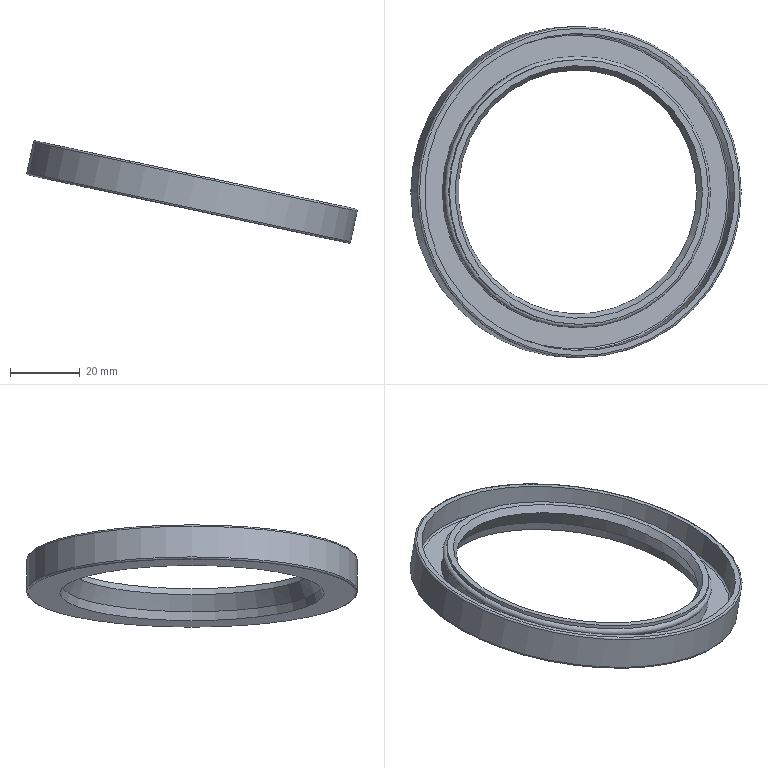Part | STEP file | HL4GZ-1.862.553 (cutter mechanism oil seal) | 1 solid | 15 faces | box 94.817 x 95 x 29.347 mm | volume 14495 mm3 | cone 4 | plane 4 | torus 4 | cylinder 3 | commonest cylinder face diameters 76 x1 91 x1 95 x1
STEP:
#1=CARTESIAN_POINT('',(0.,0.,0.));
#2=DIRECTION('',(0.,0.,1.));
#3=DIRECTION('',(1.,0.,0.));
#4=AXIS2_PLACEMENT_3D('',#1,#2,#3);
#5=CARTESIAN_POINT('',(1986.995,0.00003081,-489.503));
#6=VERTEX_POINT('',#5);
#7=CARTESIAN_POINT('',(1949.826,0.00003081,-481.603));
#8=DIRECTION('',(0.2079,0.,0.9781));
#9=DIRECTION('',(0.9781,0.,-0.2079));
#10=AXIS2_PLACEMENT_3D('',#7,#8,#9);
#11=CIRCLE('',#10,38.);
#12=CARTESIAN_POINT('',(1949.93,0.00003081,-481.114));
#13=DIRECTION('',(0.2079,0.,0.9781));
#14=DIRECTION('',(0.9781,0.,-0.2079));
#15=AXIS2_PLACEMENT_3D('',#12,#13,#14);
#16=CYLINDRICAL_SURFACE('',#15,38.);
#17=CARTESIAN_POINT('',(0.,-0.5));
#18=DIRECTION('',(1.,0.));
#19=VECTOR('',#18,1.);
#20=LINE('',#17,#19);
#21=(GEOMETRIC_REPRESENTATION_CONTEXT(2)PARAMETRIC_REPRESENTATION_CONTEXT()REPRESENTATION_CONTEXT('',''));
#22=DEFINITIONAL_REPRESENTATION('',(#20),#21);
#23=PCURVE('',#16,#22);
#24=CARTESIAN_POINT('',(1949.618,0.00003081,-482.581));
#25=DIRECTION('',(0.2079,0.,0.9781));
#26=DIRECTION('',(0.,-1.,0.));
#27=AXIS2_PLACEMENT_3D('',#24,#25,#26);
#28=TOROIDAL_SURFACE('',#27,38.,1.);
#29=CARTESIAN_POINT('',(1.571,7.854));
#30=DIRECTION('',(1.,0.));
#31=VECTOR('',#30,1.);
#32=LINE('',#29,#31);
#33=(GEOMETRIC_REPRESENTATION_CONTEXT(2)PARAMETRIC_REPRESENTATION_CONTEXT()REPRESENTATION_CONTEXT('',''));
#34=DEFINITIONAL_REPRESENTATION('',(#32),#33);
#35=PCURVE('',#28,#34);
#36=SURFACE_CURVE('',#11,(#23,#35),.PCURVE_S1.);
#37=EDGE_CURVE('',#6,#6,#36,.T.);
#38=ORIENTED_EDGE('',*,*,#37,.T.);
#39=CARTESIAN_POINT('',(1987.203,0.00003081,-488.525));
#40=VERTEX_POINT('',#39);
#41=CARTESIAN_POINT('',(1986.995,0.00003081,-489.503));
#42=CARTESIAN_POINT('',(1987.203,0.00003081,-488.525));
#43=B_SPLINE_CURVE_WITH_KNOTS('',1,(#41,#42),.UNSPECIFIED.,.F.,.F.,(2,2),(-0.5,0.5),.PIECEWISE_BEZIER_KNOTS.);
#44=CARTESIAN_POINT('',(6.283,0.));
#45=DIRECTION('',(0.,1.));
#46=VECTOR('',#45,1.);
#47=LINE('',#44,#46);
#48=(GEOMETRIC_REPRESENTATION_CONTEXT(2)PARAMETRIC_REPRESENTATION_CONTEXT()REPRESENTATION_CONTEXT('',''));
#49=DEFINITIONAL_REPRESENTATION('',(#47),#48);
#50=PCURVE('',#16,#49);
#51=CARTESIAN_POINT('',(0.,0.));
#52=DIRECTION('',(0.,1.));
#53=VECTOR('',#52,1.);
#54=LINE('',#51,#53);
#55=(GEOMETRIC_REPRESENTATION_CONTEXT(2)PARAMETRIC_REPRESENTATION_CONTEXT()REPRESENTATION_CONTEXT('',''));
#56=DEFINITIONAL_REPRESENTATION('',(#54),#55);
#57=PCURVE('',#16,#56);
#58=SEAM_CURVE('',#43,(#50,#57),.PCURVE_S1.);
#59=EDGE_CURVE('',#6,#40,#58,.T.);
#60=ORIENTED_EDGE('',*,*,#59,.T.);
#61=CARTESIAN_POINT('',(1950.034,0.00003081,-480.624));
#62=DIRECTION('',(0.2079,0.,0.9781));
#63=DIRECTION('',(0.9781,0.,-0.2079));
#64=AXIS2_PLACEMENT_3D('',#61,#62,#63);
#65=CIRCLE('',#64,38.);
#66=CARTESIAN_POINT('',(0.,0.5));
#67=DIRECTION('',(1.,0.));
#68=VECTOR('',#67,1.);
#69=LINE('',#66,#68);
#70=(GEOMETRIC_REPRESENTATION_CONTEXT(2)PARAMETRIC_REPRESENTATION_CONTEXT()REPRESENTATION_CONTEXT('',''));
#71=DEFINITIONAL_REPRESENTATION('',(#69),#70);
#72=PCURVE('',#16,#71);
#73=CARTESIAN_POINT('',(1986.347,0.00003081,-488.343));
#74=DIRECTION('',(0.2079,0.,0.9781));
#75=DIRECTION('',(0.,-1.,0.));
#76=AXIS2_PLACEMENT_3D('',#73,#74,#75);
#77=PLANE('',#76);
#78=CARTESIAN_POINT('',(0.,-37.125));
#79=DIRECTION('',(0.,1.));
#80=AXIS2_PLACEMENT_2D('',#78,#79);
#81=CIRCLE('',#80,38.);
#82=(GEOMETRIC_REPRESENTATION_CONTEXT(2)PARAMETRIC_REPRESENTATION_CONTEXT()REPRESENTATION_CONTEXT('',''));
#83=DEFINITIONAL_REPRESENTATION('',(#81),#82);
#84=PCURVE('',#77,#83);
#85=SURFACE_CURVE('',#65,(#72,#84),.PCURVE_S1.);
#86=EDGE_CURVE('',#40,#40,#85,.T.);
#87=ORIENTED_EDGE('',*,*,#86,.F.);
#88=ORIENTED_EDGE('',*,*,#59,.F.);
#89=EDGE_LOOP('',(#38,#60,#87,#88));
#90=FACE_BOUND('',#89,.T.);
#91=ADVANCED_FACE('',(#90),#16,.T.);
#92=CARTESIAN_POINT('',(1986.537,0.00003081,-495.029));
#93=VERTEX_POINT('',#92);
#94=CARTESIAN_POINT('',(1948.682,0.00003081,-486.982));
#95=DIRECTION('',(0.2079,0.,0.9781));
#96=DIRECTION('',(0.9781,0.,-0.2079));
#97=AXIS2_PLACEMENT_3D('',#94,#95,#96);
#98=CIRCLE('',#97,38.7);
#99=CARTESIAN_POINT('',(1949.046,0.00003081,-485.271));
#100=DIRECTION('',(-0.2079,0.,-0.9781));
#101=DIRECTION('',(0.9781,0.,-0.2079));
#102=AXIS2_PLACEMENT_3D('',#99,#100,#101);
#103=CONICAL_SURFACE('',#102,38.35,0.1974);
#104=CARTESIAN_POINT('',(6.283,1.75));
#105=DIRECTION('',(-1.,0.));
#106=VECTOR('',#105,1.);
#107=LINE('',#104,#106);
#108=(GEOMETRIC_REPRESENTATION_CONTEXT(2)PARAMETRIC_REPRESENTATION_CONTEXT()REPRESENTATION_CONTEXT('',''));
#109=DEFINITIONAL_REPRESENTATION('',(#107),#108);
#110=PCURVE('',#103,#109);
#111=CARTESIAN_POINT('',(1989.862,0.00003081,-495.736));
#112=DIRECTION('',(0.2079,0.,0.9781));
#113=DIRECTION('',(0.,-1.,0.));
#114=AXIS2_PLACEMENT_3D('',#111,#112,#113);
#115=PLANE('',#114);
#116=CARTESIAN_POINT('',(0.,-42.1));
#117=DIRECTION('',(0.,1.));
#118=AXIS2_PLACEMENT_2D('',#116,#117);
#119=CIRCLE('',#118,38.7);
#120=(GEOMETRIC_REPRESENTATION_CONTEXT(2)PARAMETRIC_REPRESENTATION_CONTEXT()REPRESENTATION_CONTEXT('',''));
#121=DEFINITIONAL_REPRESENTATION('',(#119),#120);
#122=PCURVE('',#115,#121);
#123=SURFACE_CURVE('',#98,(#110,#122),.PCURVE_S1.);
#124=EDGE_CURVE('',#93,#93,#123,.T.);
#125=ORIENTED_EDGE('',*,*,#124,.T.);
#126=CARTESIAN_POINT('',(1986.58,0.00003081,-491.46));
#127=VERTEX_POINT('',#126);
#128=CARTESIAN_POINT('',(1986.58,0.00003081,-491.46));
#129=CARTESIAN_POINT('',(1986.537,0.00003081,-495.029));
#130=B_SPLINE_CURVE_WITH_KNOTS('',1,(#128,#129),.UNSPECIFIED.,.F.,.F.,(2,2),(-1.785,1.785),.PIECEWISE_BEZIER_KNOTS.);
#131=CARTESIAN_POINT('',(0.,0.));
#132=DIRECTION('',(0.,1.));
#133=VECTOR('',#132,1.);
#134=LINE('',#131,#133);
#135=(GEOMETRIC_REPRESENTATION_CONTEXT(2)PARAMETRIC_REPRESENTATION_CONTEXT()REPRESENTATION_CONTEXT('',''));
#136=DEFINITIONAL_REPRESENTATION('',(#134),#135);
#137=PCURVE('',#103,#136);
#138=CARTESIAN_POINT('',(6.283,0.));
#139=DIRECTION('',(0.,1.));
#140=VECTOR('',#139,1.);
#141=LINE('',#138,#140);
#142=(GEOMETRIC_REPRESENTATION_CONTEXT(2)PARAMETRIC_REPRESENTATION_CONTEXT()REPRESENTATION_CONTEXT('',''));
#143=DEFINITIONAL_REPRESENTATION('',(#141),#142);
#144=PCURVE('',#103,#143);
#145=SEAM_CURVE('',#130,(#137,#144),.PCURVE_S1.);
#146=EDGE_CURVE('',#127,#93,#145,.T.);
#147=ORIENTED_EDGE('',*,*,#146,.F.);
#148=CARTESIAN_POINT('',(1949.41,0.00003081,-483.559));
#149=DIRECTION('',(0.2079,0.,0.9781));
#150=DIRECTION('',(0.9781,0.,-0.2079));
#151=AXIS2_PLACEMENT_3D('',#148,#149,#150);
#152=CIRCLE('',#151,38.);
#153=CARTESIAN_POINT('',(6.283,-1.75));
#154=DIRECTION('',(-1.,0.));
#155=VECTOR('',#154,1.);
#156=LINE('',#153,#155);
#157=(GEOMETRIC_REPRESENTATION_CONTEXT(2)PARAMETRIC_REPRESENTATION_CONTEXT()REPRESENTATION_CONTEXT('',''));
#158=DEFINITIONAL_REPRESENTATION('',(#156),#157);
#159=PCURVE('',#103,#158);
#160=CARTESIAN_POINT('',(1.571,4.712));
#161=DIRECTION('',(1.,0.));
#162=VECTOR('',#161,1.);
#163=LINE('',#160,#162);
#164=(GEOMETRIC_REPRESENTATION_CONTEXT(2)PARAMETRIC_REPRESENTATION_CONTEXT()REPRESENTATION_CONTEXT('',''));
#165=DEFINITIONAL_REPRESENTATION('',(#163),#164);
#166=PCURVE('',#28,#165);
#167=SURFACE_CURVE('',#152,(#159,#166),.PCURVE_S1.);
#168=EDGE_CURVE('',#127,#127,#167,.T.);
#169=ORIENTED_EDGE('',*,*,#168,.F.);
#170=ORIENTED_EDGE('',*,*,#146,.T.);
#171=EDGE_LOOP('',(#125,#147,#169,#170));
#172=FACE_BOUND('',#171,.T.);
#173=ADVANCED_FACE('',(#172),#103,.T.);
#174=CARTESIAN_POINT('',(1985.363,0.00003081,-494.779));
#175=VERTEX_POINT('',#174);
#176=CARTESIAN_POINT('',(1948.682,0.00003081,-486.982));
#177=DIRECTION('',(0.2079,0.,0.9781));
#178=DIRECTION('',(0.9781,0.,-0.2079));
#179=AXIS2_PLACEMENT_3D('',#176,#177,#178);
#180=CIRCLE('',#179,37.5);
#181=CARTESIAN_POINT('',(1948.422,0.00003081,-488.205));
#182=DIRECTION('',(-0.2079,0.,-0.9781));
#183=DIRECTION('',(0.9781,0.,-0.2079));
#184=AXIS2_PLACEMENT_3D('',#181,#182,#183);
#185=CONICAL_SURFACE('',#184,37.75,0.1974);
#186=CARTESIAN_POINT('',(6.283,-1.25));
#187=DIRECTION('',(-1.,0.));
#188=VECTOR('',#187,1.);
#189=LINE('',#186,#188);
#190=(GEOMETRIC_REPRESENTATION_CONTEXT(2)PARAMETRIC_REPRESENTATION_CONTEXT()REPRESENTATION_CONTEXT('',''));
#191=DEFINITIONAL_REPRESENTATION('',(#189),#190);
#192=PCURVE('',#185,#191);
#193=CARTESIAN_POINT('',(1949.15,0.00003081,-484.782));
#194=DIRECTION('',(-0.2079,0.,-0.9781));
#195=DIRECTION('',(0.9781,0.,-0.2079));
#196=AXIS2_PLACEMENT_3D('',#193,#194,#195);
#197=CONICAL_SURFACE('',#196,36.25,0.5071);
#198=CARTESIAN_POINT('',(6.283,2.25));
#199=DIRECTION('',(-1.,0.));
#200=VECTOR('',#199,1.);
#201=LINE('',#198,#200);
#202=(GEOMETRIC_REPRESENTATION_CONTEXT(2)PARAMETRIC_REPRESENTATION_CONTEXT()REPRESENTATION_CONTEXT('',''));
#203=DEFINITIONAL_REPRESENTATION('',(#201),#202);
#204=PCURVE('',#197,#203);
#205=SURFACE_CURVE('',#180,(#192,#204),.PCURVE_S1.);
#206=EDGE_CURVE('',#175,#175,#205,.T.);
#207=ORIENTED_EDGE('',*,*,#206,.F.);
#208=CARTESIAN_POINT('',(1985.332,0.00003081,-497.328));
#209=VERTEX_POINT('',#208);
#210=CARTESIAN_POINT('',(1985.363,0.00003081,-494.779));
#211=CARTESIAN_POINT('',(1985.332,0.00003081,-497.328));
#212=B_SPLINE_CURVE_WITH_KNOTS('',1,(#210,#211),.UNSPECIFIED.,.F.,.F.,(2,2),(-1.275,1.275),.PIECEWISE_BEZIER_KNOTS.);
#213=CARTESIAN_POINT('',(6.283,0.));
#214=DIRECTION('',(0.,1.));
#215=VECTOR('',#214,1.);
#216=LINE('',#213,#215);
#217=(GEOMETRIC_REPRESENTATION_CONTEXT(2)PARAMETRIC_REPRESENTATION_CONTEXT()REPRESENTATION_CONTEXT('',''));
#218=DEFINITIONAL_REPRESENTATION('',(#216),#217);
#219=PCURVE('',#185,#218);
#220=CARTESIAN_POINT('',(0.,0.));
#221=DIRECTION('',(0.,1.));
#222=VECTOR('',#221,1.);
#223=LINE('',#220,#222);
#224=(GEOMETRIC_REPRESENTATION_CONTEXT(2)PARAMETRIC_REPRESENTATION_CONTEXT()REPRESENTATION_CONTEXT('',''));
#225=DEFINITIONAL_REPRESENTATION('',(#223),#224);
#226=PCURVE('',#185,#225);
#227=SEAM_CURVE('',#212,(#219,#226),.PCURVE_S1.);
#228=EDGE_CURVE('',#175,#209,#227,.T.);
#229=ORIENTED_EDGE('',*,*,#228,.T.);
#230=CARTESIAN_POINT('',(1948.163,0.00003081,-489.428));
#231=DIRECTION('',(0.2079,0.,0.9781));
#232=DIRECTION('',(0.9781,0.,-0.2079));
#233=AXIS2_PLACEMENT_3D('',#230,#231,#232);
#234=CIRCLE('',#233,38.);
#235=CARTESIAN_POINT('',(6.283,1.25));
#236=DIRECTION('',(-1.,0.));
#237=VECTOR('',#236,1.);
#238=LINE('',#235,#237);
#239=(GEOMETRIC_REPRESENTATION_CONTEXT(2)PARAMETRIC_REPRESENTATION_CONTEXT()REPRESENTATION_CONTEXT('',''));
#240=DEFINITIONAL_REPRESENTATION('',(#238),#239);
#241=PCURVE('',#185,#240);
#242=CARTESIAN_POINT('',(1989.978,0.00003081,-498.316));
#243=DIRECTION('',(-0.2079,0.,-0.9781));
#244=DIRECTION('',(0.,1.,0.));
#245=AXIS2_PLACEMENT_3D('',#242,#243,#244);
#246=PLANE('',#245);
#247=CARTESIAN_POINT('',(0.,-4.75));
#248=CARTESIAN_POINT('',(65.818,-4.75));
#249=CARTESIAN_POINT('',(32.909,-61.75));
#250=CARTESIAN_POINT('',(0.,-118.75));
#251=CARTESIAN_POINT('',(-32.909,-61.75));
#252=CARTESIAN_POINT('',(-65.818,-4.75));
#253=CARTESIAN_POINT('',(0.,-4.75));
#254=(BOUNDED_CURVE()B_SPLINE_CURVE(2,(#247,#248,#249,#250,#251,#252,#253),.UNSPECIFIED.,.T.,.F.)B_SPLINE_CURVE_WITH_KNOTS((1,2,2,2,2,1),(-2.094,0.,2.094,4.189,6.283,8.378),.UNSPECIFIED.)CURVE()GEOMETRIC_REPRESENTATION_ITEM()RATIONAL_B_SPLINE_CURVE((1.,0.5,1.,0.5,1.,0.5,1.))REPRESENTATION_ITEM(''));
#255=(GEOMETRIC_REPRESENTATION_CONTEXT(2)PARAMETRIC_REPRESENTATION_CONTEXT()REPRESENTATION_CONTEXT('',''));
#256=DEFINITIONAL_REPRESENTATION('',(#254),#255);
#257=PCURVE('',#246,#256);
#258=SURFACE_CURVE('',#234,(#241,#257),.PCURVE_S1.);
#259=EDGE_CURVE('',#209,#209,#258,.T.);
#260=ORIENTED_EDGE('',*,*,#259,.T.);
#261=ORIENTED_EDGE('',*,*,#228,.F.);
#262=EDGE_LOOP('',(#207,#229,#260,#261));
#263=FACE_BOUND('',#262,.F.);
#264=ADVANCED_FACE('',(#263),#185,.F.);
#265=CARTESIAN_POINT('',(1983.853,0.00003081,-489.858));
#266=VERTEX_POINT('',#265);
#267=CARTESIAN_POINT('',(1949.618,0.00003081,-482.581));
#268=DIRECTION('',(0.2079,0.,0.9781));
#269=DIRECTION('',(0.9781,0.,-0.2079));
#270=AXIS2_PLACEMENT_3D('',#267,#268,#269);
#271=CIRCLE('',#270,35.);
#272=CARTESIAN_POINT('',(6.283,-2.25));
#273=DIRECTION('',(-1.,0.));
#274=VECTOR('',#273,1.);
#275=LINE('',#272,#274);
#276=(GEOMETRIC_REPRESENTATION_CONTEXT(2)PARAMETRIC_REPRESENTATION_CONTEXT()REPRESENTATION_CONTEXT('',''));
#277=DEFINITIONAL_REPRESENTATION('',(#275),#276);
#278=PCURVE('',#197,#277);
#279=CARTESIAN_POINT('',(1949.826,0.00003081,-481.603));
#280=DIRECTION('',(0.2079,0.,0.9781));
#281=DIRECTION('',(0.9781,0.,-0.2079));
#282=AXIS2_PLACEMENT_3D('',#279,#280,#281);
#283=CONICAL_SURFACE('',#282,35.625,0.5586);
#284=CARTESIAN_POINT('',(0.,-1.));
#285=DIRECTION('',(1.,0.));
#286=VECTOR('',#285,1.);
#287=LINE('',#284,#286);
#288=(GEOMETRIC_REPRESENTATION_CONTEXT(2)PARAMETRIC_REPRESENTATION_CONTEXT()REPRESENTATION_CONTEXT('',''));
#289=DEFINITIONAL_REPRESENTATION('',(#287),#288);
#290=PCURVE('',#283,#289);
#291=SURFACE_CURVE('',#271,(#278,#290),.PCURVE_S1.);
#292=EDGE_CURVE('',#266,#266,#291,.T.);
#293=ORIENTED_EDGE('',*,*,#292,.F.);
#294=CARTESIAN_POINT('',(1983.853,0.00003081,-489.858));
#295=CARTESIAN_POINT('',(1985.363,0.00003081,-494.779));
#296=B_SPLINE_CURVE_WITH_KNOTS('',1,(#294,#295),.UNSPECIFIED.,.F.,.F.,(2,2),(-2.574,2.574),.PIECEWISE_BEZIER_KNOTS.);
#297=CARTESIAN_POINT('',(6.283,0.));
#298=DIRECTION('',(0.,1.));
#299=VECTOR('',#298,1.);
#300=LINE('',#297,#299);
#301=(GEOMETRIC_REPRESENTATION_CONTEXT(2)PARAMETRIC_REPRESENTATION_CONTEXT()REPRESENTATION_CONTEXT('',''));
#302=DEFINITIONAL_REPRESENTATION('',(#300),#301);
#303=PCURVE('',#197,#302);
#304=CARTESIAN_POINT('',(0.,0.));
#305=DIRECTION('',(0.,1.));
#306=VECTOR('',#305,1.);
#307=LINE('',#304,#306);
#308=(GEOMETRIC_REPRESENTATION_CONTEXT(2)PARAMETRIC_REPRESENTATION_CONTEXT()REPRESENTATION_CONTEXT('',''));
#309=DEFINITIONAL_REPRESENTATION('',(#307),#308);
#310=PCURVE('',#197,#309);
#311=SEAM_CURVE('',#296,(#303,#310),.PCURVE_S1.);
#312=EDGE_CURVE('',#266,#175,#311,.T.);
#313=ORIENTED_EDGE('',*,*,#312,.T.);
#314=ORIENTED_EDGE('',*,*,#206,.T.);
#315=ORIENTED_EDGE('',*,*,#312,.F.);
#316=EDGE_LOOP('',(#293,#313,#314,#315));
#317=FACE_BOUND('',#316,.F.);
#318=ADVANCED_FACE('',(#317),#197,.F.);
#319=CARTESIAN_POINT('',(1985.492,0.00003081,-488.161));
#320=VERTEX_POINT('',#319);
#321=CARTESIAN_POINT('',(1950.034,0.00003081,-480.624));
#322=DIRECTION('',(0.2079,0.,0.9781));
#323=DIRECTION('',(0.9781,0.,-0.2079));
#324=AXIS2_PLACEMENT_3D('',#321,#322,#323);
#325=CIRCLE('',#324,36.25);
#326=CARTESIAN_POINT('',(0.,1.));
#327=DIRECTION('',(1.,0.));
#328=VECTOR('',#327,1.);
#329=LINE('',#326,#328);
#330=(GEOMETRIC_REPRESENTATION_CONTEXT(2)PARAMETRIC_REPRESENTATION_CONTEXT()REPRESENTATION_CONTEXT('',''));
#331=DEFINITIONAL_REPRESENTATION('',(#329),#330);
#332=PCURVE('',#283,#331);
#333=CARTESIAN_POINT('',(0.,-37.125));
#334=DIRECTION('',(0.,1.));
#335=AXIS2_PLACEMENT_2D('',#333,#334);
#336=CIRCLE('',#335,36.25);
#337=(GEOMETRIC_REPRESENTATION_CONTEXT(2)PARAMETRIC_REPRESENTATION_CONTEXT()REPRESENTATION_CONTEXT('',''));
#338=DEFINITIONAL_REPRESENTATION('',(#336),#337);
#339=PCURVE('',#77,#338);
#340=SURFACE_CURVE('',#325,(#332,#339),.PCURVE_S1.);
#341=EDGE_CURVE('',#320,#320,#340,.T.);
#342=ORIENTED_EDGE('',*,*,#341,.F.);
#343=CARTESIAN_POINT('',(1983.853,0.00003081,-489.858));
#344=CARTESIAN_POINT('',(1985.492,0.00003081,-488.161));
#345=B_SPLINE_CURVE_WITH_KNOTS('',1,(#343,#344),.UNSPECIFIED.,.F.,.F.,(2,2),(-1.179,1.179),.PIECEWISE_BEZIER_KNOTS.);
#346=CARTESIAN_POINT('',(0.,0.));
#347=DIRECTION('',(0.,1.));
#348=VECTOR('',#347,1.);
#349=LINE('',#346,#348);
#350=(GEOMETRIC_REPRESENTATION_CONTEXT(2)PARAMETRIC_REPRESENTATION_CONTEXT()REPRESENTATION_CONTEXT('',''));
#351=DEFINITIONAL_REPRESENTATION('',(#349),#350);
#352=PCURVE('',#283,#351);
#353=CARTESIAN_POINT('',(6.283,0.));
#354=DIRECTION('',(0.,1.));
#355=VECTOR('',#354,1.);
#356=LINE('',#353,#355);
#357=(GEOMETRIC_REPRESENTATION_CONTEXT(2)PARAMETRIC_REPRESENTATION_CONTEXT()REPRESENTATION_CONTEXT('',''));
#358=DEFINITIONAL_REPRESENTATION('',(#356),#357);
#359=PCURVE('',#283,#358);
#360=SEAM_CURVE('',#345,(#352,#359),.PCURVE_S1.);
#361=EDGE_CURVE('',#266,#320,#360,.T.);
#362=ORIENTED_EDGE('',*,*,#361,.F.);
#363=ORIENTED_EDGE('',*,*,#292,.T.);
#364=ORIENTED_EDGE('',*,*,#361,.T.);
#365=EDGE_LOOP('',(#342,#362,#363,#364));
#366=FACE_BOUND('',#365,.F.);
#367=ADVANCED_FACE('',(#366),#283,.F.);
#368=ORIENTED_EDGE('',*,*,#341,.F.);
#369=EDGE_LOOP('',(#368));
#370=FACE_BOUND('',#369,.T.);
#371=ORIENTED_EDGE('',*,*,#86,.T.);
#372=EDGE_LOOP('',(#371));
#373=FACE_BOUND('',#372,.T.);
#374=ADVANCED_FACE('',(#370,#373),#77,.T.);
#375=ORIENTED_EDGE('',*,*,#37,.F.);
#376=CARTESIAN_POINT('',(1986.58,0.00003081,-491.46));
#377=CARTESIAN_POINT('',(1986.964,0.00003081,-491.541));
#378=CARTESIAN_POINT('',(1987.384,0.00003081,-491.45));
#379=CARTESIAN_POINT('',(1987.752,0.00003081,-491.168));
#380=CARTESIAN_POINT('',(1987.963,0.00003081,-490.731));
#381=CARTESIAN_POINT('',(1987.948,0.00003081,-490.246));
#382=CARTESIAN_POINT('',(1987.727,0.00003081,-489.839));
#383=CARTESIAN_POINT('',(1987.38,0.00003081,-489.585));
#384=CARTESIAN_POINT('',(1986.995,0.00003081,-489.503));
#385=B_SPLINE_CURVE_WITH_KNOTS('',8,(#376,#377,#378,#379,#380,#381,#382,#383,#384),.UNSPECIFIED.,.F.,.F.,(9,9),(-1.571,1.571),.PIECEWISE_BEZIER_KNOTS.);
#386=CARTESIAN_POINT('',(1.571,6.283));
#387=DIRECTION('',(0.,1.));
#388=VECTOR('',#387,1.);
#389=LINE('',#386,#388);
#390=(GEOMETRIC_REPRESENTATION_CONTEXT(2)PARAMETRIC_REPRESENTATION_CONTEXT()REPRESENTATION_CONTEXT('',''));
#391=DEFINITIONAL_REPRESENTATION('',(#389),#390);
#392=PCURVE('',#28,#391);
#393=CARTESIAN_POINT('',(7.854,6.283));
#394=DIRECTION('',(0.,1.));
#395=VECTOR('',#394,1.);
#396=LINE('',#393,#395);
#397=(GEOMETRIC_REPRESENTATION_CONTEXT(2)PARAMETRIC_REPRESENTATION_CONTEXT()REPRESENTATION_CONTEXT('',''));
#398=DEFINITIONAL_REPRESENTATION('',(#396),#397);
#399=PCURVE('',#28,#398);
#400=SEAM_CURVE('',#385,(#392,#399),.PCURVE_S1.);
#401=EDGE_CURVE('',#127,#6,#400,.T.);
#402=ORIENTED_EDGE('',*,*,#401,.F.);
#403=ORIENTED_EDGE('',*,*,#168,.T.);
#404=ORIENTED_EDGE('',*,*,#401,.T.);
#405=EDGE_LOOP('',(#375,#402,#403,#404));
#406=FACE_BOUND('',#405,.T.);
#407=ADVANCED_FACE('',(#406),#28,.T.);
#408=CARTESIAN_POINT('',(1994.747,0.00003081,-489.106));
#409=VERTEX_POINT('',#408);
#410=CARTESIAN_POINT('',(1950.242,0.00003081,-479.646));
#411=DIRECTION('',(0.2079,0.,0.9781));
#412=DIRECTION('',(0.9781,0.,-0.2079));
#413=AXIS2_PLACEMENT_3D('',#410,#411,#412);
#414=CIRCLE('',#413,45.5);
#415=CARTESIAN_POINT('',(1995.725,0.00003081,-489.314));
#416=DIRECTION('',(0.2079,0.,0.9781));
#417=DIRECTION('',(0.,-1.,0.));
#418=AXIS2_PLACEMENT_3D('',#415,#416,#417);
#419=PLANE('',#418);
#420=CARTESIAN_POINT('',(0.,-46.5));
#421=DIRECTION('',(0.,1.));
#422=AXIS2_PLACEMENT_2D('',#420,#421);
#423=CIRCLE('',#422,45.5);
#424=(GEOMETRIC_REPRESENTATION_CONTEXT(2)PARAMETRIC_REPRESENTATION_CONTEXT()REPRESENTATION_CONTEXT('',''));
#425=DEFINITIONAL_REPRESENTATION('',(#423),#424);
#426=PCURVE('',#419,#425);
#427=CARTESIAN_POINT('',(1949.462,0.00003081,-483.314));
#428=DIRECTION('',(0.2079,0.,0.9781));
#429=DIRECTION('',(0.9781,0.,-0.2079));
#430=AXIS2_PLACEMENT_3D('',#427,#428,#429);
#431=CYLINDRICAL_SURFACE('',#430,45.5);
#432=CARTESIAN_POINT('',(0.,3.75));
#433=DIRECTION('',(1.,0.));
#434=VECTOR('',#433,1.);
#435=LINE('',#432,#434);
#436=(GEOMETRIC_REPRESENTATION_CONTEXT(2)PARAMETRIC_REPRESENTATION_CONTEXT()REPRESENTATION_CONTEXT('',''));
#437=DEFINITIONAL_REPRESENTATION('',(#435),#436);
#438=PCURVE('',#431,#437);
#439=SURFACE_CURVE('',#414,(#426,#438),.PCURVE_S1.);
#440=EDGE_CURVE('',#409,#409,#439,.T.);
#441=ORIENTED_EDGE('',*,*,#440,.F.);
#442=EDGE_LOOP('',(#441));
#443=FACE_BOUND('',#442,.T.);
#444=CARTESIAN_POINT('',(1996.215,0.00003081,-489.418));
#445=VERTEX_POINT('',#444);
#446=CARTESIAN_POINT('',(1950.242,0.00003081,-479.646));
#447=DIRECTION('',(-0.2079,0.,-0.9781));
#448=DIRECTION('',(-0.9781,0.,0.2079));
#449=AXIS2_PLACEMENT_3D('',#446,#447,#448);
#450=CIRCLE('',#449,47.);
#451=CARTESIAN_POINT('',(0.,-93.5));
#452=CARTESIAN_POINT('',(-81.406,-93.5));
#453=CARTESIAN_POINT('',(-40.703,-23.));
#454=CARTESIAN_POINT('',(0.,47.5));
#455=CARTESIAN_POINT('',(40.703,-23.));
#456=CARTESIAN_POINT('',(81.406,-93.5));
#457=CARTESIAN_POINT('',(0.,-93.5));
#458=(BOUNDED_CURVE()B_SPLINE_CURVE(2,(#451,#452,#453,#454,#455,#456,#457),.UNSPECIFIED.,.T.,.F.)B_SPLINE_CURVE_WITH_KNOTS((1,2,2,2,2,1),(-2.094,0.,2.094,4.189,6.283,8.378),.UNSPECIFIED.)CURVE()GEOMETRIC_REPRESENTATION_ITEM()RATIONAL_B_SPLINE_CURVE((1.,0.5,1.,0.5,1.,0.5,1.))REPRESENTATION_ITEM(''));
#459=(GEOMETRIC_REPRESENTATION_CONTEXT(2)PARAMETRIC_REPRESENTATION_CONTEXT()REPRESENTATION_CONTEXT('',''));
#460=DEFINITIONAL_REPRESENTATION('',(#458),#459);
#461=PCURVE('',#419,#460);
#462=CARTESIAN_POINT('',(1950.138,0.00003081,-480.135));
#463=DIRECTION('',(0.2079,0.,0.9781));
#464=DIRECTION('',(0.,-1.,0.));
#465=AXIS2_PLACEMENT_3D('',#462,#463,#464);
#466=TOROIDAL_SURFACE('',#465,47.,0.5);
#467=CARTESIAN_POINT('',(10.996,7.854));
#468=DIRECTION('',(-1.,0.));
#469=VECTOR('',#468,1.);
#470=LINE('',#467,#469);
#471=(GEOMETRIC_REPRESENTATION_CONTEXT(2)PARAMETRIC_REPRESENTATION_CONTEXT()REPRESENTATION_CONTEXT('',''));
#472=DEFINITIONAL_REPRESENTATION('',(#470),#471);
#473=PCURVE('',#466,#472);
#474=SURFACE_CURVE('',#450,(#461,#473),.PCURVE_S1.);
#475=EDGE_CURVE('',#445,#445,#474,.T.);
#476=ORIENTED_EDGE('',*,*,#475,.F.);
#477=EDGE_LOOP('',(#476));
#478=FACE_BOUND('',#477,.T.);
#479=ADVANCED_FACE('',(#443,#478),#419,.T.);
#480=ORIENTED_EDGE('',*,*,#475,.T.);
#481=CARTESIAN_POINT('',(1996.6,0.00003081,-490.011));
#482=VERTEX_POINT('',#481);
#483=CARTESIAN_POINT('',(1996.6,0.00003081,-490.011));
#484=CARTESIAN_POINT('',(1996.627,0.00003081,-489.88));
#485=CARTESIAN_POINT('',(1996.613,0.00003081,-489.744));
#486=CARTESIAN_POINT('',(1996.557,0.00003081,-489.618));
#487=CARTESIAN_POINT('',(1996.464,0.00003081,-489.515));
#488=CARTESIAN_POINT('',(1996.345,0.00003081,-489.446));
#489=CARTESIAN_POINT('',(1996.215,0.00003081,-489.418));
#490=(BOUNDED_CURVE()B_SPLINE_CURVE(6,(#483,#484,#485,#486,#487,#488,#489),.UNSPECIFIED.,.F.,.F.)B_SPLINE_CURVE_WITH_KNOTS((7,7),(0.,1.571),.PIECEWISE_BEZIER_KNOTS.)CURVE()GEOMETRIC_REPRESENTATION_ITEM()RATIONAL_B_SPLINE_CURVE((1.031,1.01,0.9979,0.994,0.9979,1.01,1.031))REPRESENTATION_ITEM(''));
#491=CARTESIAN_POINT('',(1.571,6.283));
#492=DIRECTION('',(0.,1.));
#493=VECTOR('',#492,1.);
#494=LINE('',#491,#493);
#495=(GEOMETRIC_REPRESENTATION_CONTEXT(2)PARAMETRIC_REPRESENTATION_CONTEXT()REPRESENTATION_CONTEXT('',''));
#496=DEFINITIONAL_REPRESENTATION('',(#494),#495);
#497=PCURVE('',#466,#496);
#498=CARTESIAN_POINT('',(7.854,6.283));
#499=DIRECTION('',(0.,1.));
#500=VECTOR('',#499,1.);
#501=LINE('',#498,#500);
#502=(GEOMETRIC_REPRESENTATION_CONTEXT(2)PARAMETRIC_REPRESENTATION_CONTEXT()REPRESENTATION_CONTEXT('',''));
#503=DEFINITIONAL_REPRESENTATION('',(#501),#502);
#504=PCURVE('',#466,#503);
#505=SEAM_CURVE('',#490,(#497,#504),.PCURVE_S1.);
#506=EDGE_CURVE('',#482,#445,#505,.T.);
#507=ORIENTED_EDGE('',*,*,#506,.F.);
#508=CARTESIAN_POINT('',(1950.138,0.00003081,-480.135));
#509=DIRECTION('',(0.2079,0.,0.9781));
#510=DIRECTION('',(-0.9781,0.,0.2079));
#511=AXIS2_PLACEMENT_3D('',#508,#509,#510);
#512=CIRCLE('',#511,47.5);
#513=CARTESIAN_POINT('',(-1.571,6.283));
#514=DIRECTION('',(1.,0.));
#515=VECTOR('',#514,1.);
#516=LINE('',#513,#515);
#517=(GEOMETRIC_REPRESENTATION_CONTEXT(2)PARAMETRIC_REPRESENTATION_CONTEXT()REPRESENTATION_CONTEXT('',''));
#518=DEFINITIONAL_REPRESENTATION('',(#516),#517);
#519=PCURVE('',#466,#518);
#520=CARTESIAN_POINT('',(1949.202,0.00003081,-484.537));
#521=DIRECTION('',(0.2079,0.,0.9781));
#522=DIRECTION('',(0.9781,0.,-0.2079));
#523=AXIS2_PLACEMENT_3D('',#520,#521,#522);
#524=CYLINDRICAL_SURFACE('',#523,47.5);
#525=CARTESIAN_POINT('',(-3.142,4.5));
#526=DIRECTION('',(1.,0.));
#527=VECTOR('',#526,1.);
#528=LINE('',#525,#527);
#529=(GEOMETRIC_REPRESENTATION_CONTEXT(2)PARAMETRIC_REPRESENTATION_CONTEXT()REPRESENTATION_CONTEXT('',''));
#530=DEFINITIONAL_REPRESENTATION('',(#528),#529);
#531=PCURVE('',#524,#530);
#532=SURFACE_CURVE('',#512,(#519,#531),.PCURVE_S1.);
#533=EDGE_CURVE('',#482,#482,#532,.T.);
#534=ORIENTED_EDGE('',*,*,#533,.T.);
#535=ORIENTED_EDGE('',*,*,#506,.T.);
#536=EDGE_LOOP('',(#480,#507,#534,#535));
#537=FACE_BOUND('',#536,.T.);
#538=ADVANCED_FACE('',(#537),#466,.T.);
#539=ORIENTED_EDGE('',*,*,#259,.T.);
#540=EDGE_LOOP('',(#539));
#541=FACE_BOUND('',#540,.T.);
#542=CARTESIAN_POINT('',(1994.135,0.00003081,-499.2));
#543=VERTEX_POINT('',#542);
#544=CARTESIAN_POINT('',(1948.163,0.00003081,-489.428));
#545=DIRECTION('',(0.2079,0.,0.9781));
#546=DIRECTION('',(-0.9781,0.,0.2079));
#547=AXIS2_PLACEMENT_3D('',#544,#545,#546);
#548=CIRCLE('',#547,47.);
#549=CARTESIAN_POINT('',(0.,-89.75));
#550=CARTESIAN_POINT('',(-81.406,-89.75));
#551=CARTESIAN_POINT('',(-40.703,-19.25));
#552=CARTESIAN_POINT('',(0.,51.25));
#553=CARTESIAN_POINT('',(40.703,-19.25));
#554=CARTESIAN_POINT('',(81.406,-89.75));
#555=CARTESIAN_POINT('',(0.,-89.75));
#556=(BOUNDED_CURVE()B_SPLINE_CURVE(2,(#549,#550,#551,#552,#553,#554,#555),.UNSPECIFIED.,.T.,.F.)B_SPLINE_CURVE_WITH_KNOTS((1,2,2,2,2,1),(-2.094,0.,2.094,4.189,6.283,8.378),.UNSPECIFIED.)CURVE()GEOMETRIC_REPRESENTATION_ITEM()RATIONAL_B_SPLINE_CURVE((1.,0.5,1.,0.5,1.,0.5,1.))REPRESENTATION_ITEM(''));
#557=(GEOMETRIC_REPRESENTATION_CONTEXT(2)PARAMETRIC_REPRESENTATION_CONTEXT()REPRESENTATION_CONTEXT('',''));
#558=DEFINITIONAL_REPRESENTATION('',(#556),#557);
#559=PCURVE('',#246,#558);
#560=CARTESIAN_POINT('',(1948.266,0.00003081,-488.939));
#561=DIRECTION('',(0.2079,0.,0.9781));
#562=DIRECTION('',(0.,-1.,0.));
#563=AXIS2_PLACEMENT_3D('',#560,#561,#562);
#564=TOROIDAL_SURFACE('',#563,47.,0.5);
#565=CARTESIAN_POINT('',(-1.571,4.712));
#566=DIRECTION('',(1.,0.));
#567=VECTOR('',#566,1.);
#568=LINE('',#565,#567);
#569=(GEOMETRIC_REPRESENTATION_CONTEXT(2)PARAMETRIC_REPRESENTATION_CONTEXT()REPRESENTATION_CONTEXT('',''));
#570=DEFINITIONAL_REPRESENTATION('',(#568),#569);
#571=PCURVE('',#564,#570);
#572=SURFACE_CURVE('',#548,(#559,#571),.PCURVE_S1.);
#573=EDGE_CURVE('',#543,#543,#572,.T.);
#574=ORIENTED_EDGE('',*,*,#573,.F.);
#575=EDGE_LOOP('',(#574));
#576=FACE_BOUND('',#575,.T.);
#577=ADVANCED_FACE('',(#541,#576),#246,.T.);
#578=CARTESIAN_POINT('',(1994.728,0.00003081,-498.815));
#579=VERTEX_POINT('',#578);
#580=CARTESIAN_POINT('',(1948.266,0.00003081,-488.939));
#581=DIRECTION('',(-0.2079,0.,-0.9781));
#582=DIRECTION('',(-0.9781,0.,0.2079));
#583=AXIS2_PLACEMENT_3D('',#580,#581,#582);
#584=CIRCLE('',#583,47.5);
#585=CARTESIAN_POINT('',(9.425,-4.5));
#586=DIRECTION('',(-1.,0.));
#587=VECTOR('',#586,1.);
#588=LINE('',#585,#587);
#589=(GEOMETRIC_REPRESENTATION_CONTEXT(2)PARAMETRIC_REPRESENTATION_CONTEXT()REPRESENTATION_CONTEXT('',''));
#590=DEFINITIONAL_REPRESENTATION('',(#588),#589);
#591=PCURVE('',#524,#590);
#592=CARTESIAN_POINT('',(10.996,6.283));
#593=DIRECTION('',(-1.,0.));
#594=VECTOR('',#593,1.);
#595=LINE('',#592,#594);
#596=(GEOMETRIC_REPRESENTATION_CONTEXT(2)PARAMETRIC_REPRESENTATION_CONTEXT()REPRESENTATION_CONTEXT('',''));
#597=DEFINITIONAL_REPRESENTATION('',(#595),#596);
#598=PCURVE('',#564,#597);
#599=SURFACE_CURVE('',#584,(#591,#598),.PCURVE_S1.);
#600=EDGE_CURVE('',#579,#579,#599,.T.);
#601=ORIENTED_EDGE('',*,*,#600,.F.);
#602=CARTESIAN_POINT('',(1994.728,0.00003081,-498.815));
#603=CARTESIAN_POINT('',(1996.6,0.00003081,-490.011));
#604=B_SPLINE_CURVE_WITH_KNOTS('',1,(#602,#603),.UNSPECIFIED.,.F.,.F.,(2,2),(-4.5,4.5),.PIECEWISE_BEZIER_KNOTS.);
#605=CARTESIAN_POINT('',(6.283,0.));
#606=DIRECTION('',(0.,1.));
#607=VECTOR('',#606,1.);
#608=LINE('',#605,#607);
#609=(GEOMETRIC_REPRESENTATION_CONTEXT(2)PARAMETRIC_REPRESENTATION_CONTEXT()REPRESENTATION_CONTEXT('',''));
#610=DEFINITIONAL_REPRESENTATION('',(#608),#609);
#611=PCURVE('',#524,#610);
#612=CARTESIAN_POINT('',(0.,0.));
#613=DIRECTION('',(0.,1.));
#614=VECTOR('',#613,1.);
#615=LINE('',#612,#614);
#616=(GEOMETRIC_REPRESENTATION_CONTEXT(2)PARAMETRIC_REPRESENTATION_CONTEXT()REPRESENTATION_CONTEXT('',''));
#617=DEFINITIONAL_REPRESENTATION('',(#615),#616);
#618=PCURVE('',#524,#617);
#619=SEAM_CURVE('',#604,(#611,#618),.PCURVE_S1.);
#620=EDGE_CURVE('',#579,#482,#619,.T.);
#621=ORIENTED_EDGE('',*,*,#620,.T.);
#622=ORIENTED_EDGE('',*,*,#533,.F.);
#623=ORIENTED_EDGE('',*,*,#620,.F.);
#624=EDGE_LOOP('',(#601,#621,#622,#623));
#625=FACE_BOUND('',#624,.T.);
#626=ADVANCED_FACE('',(#625),#524,.T.);
#627=ORIENTED_EDGE('',*,*,#600,.T.);
#628=CARTESIAN_POINT('',(1994.135,0.00003081,-499.2));
#629=CARTESIAN_POINT('',(1994.266,0.00003081,-499.227));
#630=CARTESIAN_POINT('',(1994.402,0.00003081,-499.213));
#631=CARTESIAN_POINT('',(1994.529,0.00003081,-499.157));
#632=CARTESIAN_POINT('',(1994.632,0.00003081,-499.064));
#633=CARTESIAN_POINT('',(1994.701,0.00003081,-498.945));
#634=CARTESIAN_POINT('',(1994.728,0.00003081,-498.815));
#635=(BOUNDED_CURVE()B_SPLINE_CURVE(6,(#628,#629,#630,#631,#632,#633,#634),.UNSPECIFIED.,.F.,.F.)B_SPLINE_CURVE_WITH_KNOTS((7,7),(-1.571,0.),.PIECEWISE_BEZIER_KNOTS.)CURVE()GEOMETRIC_REPRESENTATION_ITEM()RATIONAL_B_SPLINE_CURVE((1.031,1.01,0.9979,0.994,0.9979,1.01,1.031))REPRESENTATION_ITEM(''));
#636=CARTESIAN_POINT('',(1.571,6.283));
#637=DIRECTION('',(0.,1.));
#638=VECTOR('',#637,1.);
#639=LINE('',#636,#638);
#640=(GEOMETRIC_REPRESENTATION_CONTEXT(2)PARAMETRIC_REPRESENTATION_CONTEXT()REPRESENTATION_CONTEXT('',''));
#641=DEFINITIONAL_REPRESENTATION('',(#639),#640);
#642=PCURVE('',#564,#641);
#643=CARTESIAN_POINT('',(7.854,6.283));
#644=DIRECTION('',(0.,1.));
#645=VECTOR('',#644,1.);
#646=LINE('',#643,#645);
#647=(GEOMETRIC_REPRESENTATION_CONTEXT(2)PARAMETRIC_REPRESENTATION_CONTEXT()REPRESENTATION_CONTEXT('',''));
#648=DEFINITIONAL_REPRESENTATION('',(#646),#647);
#649=PCURVE('',#564,#648);
#650=SEAM_CURVE('',#635,(#642,#649),.PCURVE_S1.);
#651=EDGE_CURVE('',#543,#579,#650,.T.);
#652=ORIENTED_EDGE('',*,*,#651,.F.);
#653=ORIENTED_EDGE('',*,*,#573,.T.);
#654=ORIENTED_EDGE('',*,*,#651,.T.);
#655=EDGE_LOOP('',(#627,#652,#653,#654));
#656=FACE_BOUND('',#655,.T.);
#657=ADVANCED_FACE('',(#656),#564,.T.);
#658=ORIENTED_EDGE('',*,*,#124,.F.);
#659=EDGE_LOOP('',(#658));
#660=FACE_BOUND('',#659,.T.);
#661=CARTESIAN_POINT('',(1992.699,0.00003081,-496.338));
#662=VERTEX_POINT('',#661);
#663=CARTESIAN_POINT('',(1948.682,0.00003081,-486.982));
#664=DIRECTION('',(-0.2079,0.,-0.9781));
#665=DIRECTION('',(-0.9781,0.,0.2079));
#666=AXIS2_PLACEMENT_3D('',#663,#664,#665);
#667=CIRCLE('',#666,45.);
#668=CARTESIAN_POINT('',(0.,-87.1));
#669=CARTESIAN_POINT('',(-77.942,-87.1));
#670=CARTESIAN_POINT('',(-38.971,-19.6));
#671=CARTESIAN_POINT('',(0.,47.9));
#672=CARTESIAN_POINT('',(38.971,-19.6));
#673=CARTESIAN_POINT('',(77.942,-87.1));
#674=CARTESIAN_POINT('',(0.,-87.1));
#675=(BOUNDED_CURVE()B_SPLINE_CURVE(2,(#668,#669,#670,#671,#672,#673,#674),.UNSPECIFIED.,.T.,.F.)B_SPLINE_CURVE_WITH_KNOTS((1,2,2,2,2,1),(-2.094,0.,2.094,4.189,6.283,8.378),.UNSPECIFIED.)CURVE()GEOMETRIC_REPRESENTATION_ITEM()RATIONAL_B_SPLINE_CURVE((1.,0.5,1.,0.5,1.,0.5,1.))REPRESENTATION_ITEM(''));
#676=(GEOMETRIC_REPRESENTATION_CONTEXT(2)PARAMETRIC_REPRESENTATION_CONTEXT()REPRESENTATION_CONTEXT('',''));
#677=DEFINITIONAL_REPRESENTATION('',(#675),#676);
#678=PCURVE('',#115,#677);
#679=CARTESIAN_POINT('',(1948.786,0.00003081,-486.493));
#680=DIRECTION('',(0.2079,0.,0.9781));
#681=DIRECTION('',(0.,-1.,0.));
#682=AXIS2_PLACEMENT_3D('',#679,#680,#681);
#683=TOROIDAL_SURFACE('',#682,45.,0.5);
#684=CARTESIAN_POINT('',(10.996,4.712));
#685=DIRECTION('',(-1.,0.));
#686=VECTOR('',#685,1.);
#687=LINE('',#684,#686);
#688=(GEOMETRIC_REPRESENTATION_CONTEXT(2)PARAMETRIC_REPRESENTATION_CONTEXT()REPRESENTATION_CONTEXT('',''));
#689=DEFINITIONAL_REPRESENTATION('',(#687),#688);
#690=PCURVE('',#683,#689);
#691=SURFACE_CURVE('',#667,(#678,#690),.PCURVE_S1.);
#692=EDGE_CURVE('',#662,#662,#691,.T.);
#693=ORIENTED_EDGE('',*,*,#692,.F.);
#694=EDGE_LOOP('',(#693));
#695=FACE_BOUND('',#694,.T.);
#696=ADVANCED_FACE('',(#660,#695),#115,.T.);
#697=CARTESIAN_POINT('',(1993.292,0.00003081,-495.953));
#698=VERTEX_POINT('',#697);
#699=CARTESIAN_POINT('',(1948.786,0.00003081,-486.493));
#700=DIRECTION('',(0.2079,0.,0.9781));
#701=DIRECTION('',(-0.9781,0.,0.2079));
#702=AXIS2_PLACEMENT_3D('',#699,#700,#701);
#703=CIRCLE('',#702,45.5);
#704=CARTESIAN_POINT('',(-3.142,-3.25));
#705=DIRECTION('',(1.,0.));
#706=VECTOR('',#705,1.);
#707=LINE('',#704,#706);
#708=(GEOMETRIC_REPRESENTATION_CONTEXT(2)PARAMETRIC_REPRESENTATION_CONTEXT()REPRESENTATION_CONTEXT('',''));
#709=DEFINITIONAL_REPRESENTATION('',(#707),#708);
#710=PCURVE('',#431,#709);
#711=CARTESIAN_POINT('',(-1.571,6.283));
#712=DIRECTION('',(1.,0.));
#713=VECTOR('',#712,1.);
#714=LINE('',#711,#713);
#715=(GEOMETRIC_REPRESENTATION_CONTEXT(2)PARAMETRIC_REPRESENTATION_CONTEXT()REPRESENTATION_CONTEXT('',''));
#716=DEFINITIONAL_REPRESENTATION('',(#714),#715);
#717=PCURVE('',#683,#716);
#718=SURFACE_CURVE('',#703,(#710,#717),.PCURVE_S1.);
#719=EDGE_CURVE('',#698,#698,#718,.T.);
#720=ORIENTED_EDGE('',*,*,#719,.T.);
#721=CARTESIAN_POINT('',(1993.292,0.00003081,-495.953));
#722=CARTESIAN_POINT('',(1994.747,0.00003081,-489.106));
#723=B_SPLINE_CURVE_WITH_KNOTS('',1,(#721,#722),.UNSPECIFIED.,.F.,.F.,(2,2),(-3.25,3.75),.PIECEWISE_BEZIER_KNOTS.);
#724=CARTESIAN_POINT('',(6.283,0.));
#725=DIRECTION('',(0.,1.));
#726=VECTOR('',#725,1.);
#727=LINE('',#724,#726);
#728=(GEOMETRIC_REPRESENTATION_CONTEXT(2)PARAMETRIC_REPRESENTATION_CONTEXT()REPRESENTATION_CONTEXT('',''));
#729=DEFINITIONAL_REPRESENTATION('',(#727),#728);
#730=PCURVE('',#431,#729);
#731=CARTESIAN_POINT('',(0.,0.));
#732=DIRECTION('',(0.,1.));
#733=VECTOR('',#732,1.);
#734=LINE('',#731,#733);
#735=(GEOMETRIC_REPRESENTATION_CONTEXT(2)PARAMETRIC_REPRESENTATION_CONTEXT()REPRESENTATION_CONTEXT('',''));
#736=DEFINITIONAL_REPRESENTATION('',(#734),#735);
#737=PCURVE('',#431,#736);
#738=SEAM_CURVE('',#723,(#730,#737),.PCURVE_S1.);
#739=EDGE_CURVE('',#698,#409,#738,.T.);
#740=ORIENTED_EDGE('',*,*,#739,.T.);
#741=ORIENTED_EDGE('',*,*,#440,.F.);
#742=ORIENTED_EDGE('',*,*,#739,.F.);
#743=EDGE_LOOP('',(#720,#740,#741,#742));
#744=FACE_BOUND('',#743,.F.);
#745=ADVANCED_FACE('',(#744),#431,.F.);
#746=ORIENTED_EDGE('',*,*,#692,.F.);
#747=CARTESIAN_POINT('',(1992.699,0.00003081,-496.338));
#748=CARTESIAN_POINT('',(1992.83,0.00003081,-496.366));
#749=CARTESIAN_POINT('',(1992.966,0.00003081,-496.352));
#750=CARTESIAN_POINT('',(1993.092,0.00003081,-496.295));
#751=CARTESIAN_POINT('',(1993.196,0.00003081,-496.203));
#752=CARTESIAN_POINT('',(1993.264,0.00003081,-496.084));
#753=CARTESIAN_POINT('',(1993.292,0.00003081,-495.953));
#754=(BOUNDED_CURVE()B_SPLINE_CURVE(6,(#747,#748,#749,#750,#751,#752,#753),.UNSPECIFIED.,.F.,.F.)B_SPLINE_CURVE_WITH_KNOTS((7,7),(4.712,6.283),.PIECEWISE_BEZIER_KNOTS.)CURVE()GEOMETRIC_REPRESENTATION_ITEM()RATIONAL_B_SPLINE_CURVE((1.031,1.01,0.9979,0.994,0.9979,1.01,1.031))REPRESENTATION_ITEM(''));
#755=CARTESIAN_POINT('',(7.854,0.));
#756=DIRECTION('',(0.,1.));
#757=VECTOR('',#756,1.);
#758=LINE('',#755,#757);
#759=(GEOMETRIC_REPRESENTATION_CONTEXT(2)PARAMETRIC_REPRESENTATION_CONTEXT()REPRESENTATION_CONTEXT('',''));
#760=DEFINITIONAL_REPRESENTATION('',(#758),#759);
#761=PCURVE('',#683,#760);
#762=CARTESIAN_POINT('',(1.571,0.));
#763=DIRECTION('',(0.,1.));
#764=VECTOR('',#763,1.);
#765=LINE('',#762,#764);
#766=(GEOMETRIC_REPRESENTATION_CONTEXT(2)PARAMETRIC_REPRESENTATION_CONTEXT()REPRESENTATION_CONTEXT('',''));
#767=DEFINITIONAL_REPRESENTATION('',(#765),#766);
#768=PCURVE('',#683,#767);
#769=SEAM_CURVE('',#754,(#761,#768),.PCURVE_S1.);
#770=EDGE_CURVE('',#662,#698,#769,.T.);
#771=ORIENTED_EDGE('',*,*,#770,.T.);
#772=ORIENTED_EDGE('',*,*,#719,.F.);
#773=ORIENTED_EDGE('',*,*,#770,.F.);
#774=EDGE_LOOP('',(#746,#771,#772,#773));
#775=FACE_BOUND('',#774,.F.);
#776=ADVANCED_FACE('',(#775),#683,.F.);
#777=CLOSED_SHELL('',(#91,#173,#264,#318,#367,#374,#407,#479,#538,#577,#626,#657,#696,#745,#776));
#778=MANIFOLD_SOLID_BREP('',#777);
#779=(LENGTH_UNIT()NAMED_UNIT(*)SI_UNIT(.MILLI.,.METRE.));
#780=UNCERTAINTY_MEASURE_WITH_UNIT(LENGTH_MEASURE(0.00001),#779,'','');
#781=(NAMED_UNIT(*)PLANE_ANGLE_UNIT()SI_UNIT($,.RADIAN.));
#782=(NAMED_UNIT(*)SI_UNIT($,.STERADIAN.)SOLID_ANGLE_UNIT());
#783=(GEOMETRIC_REPRESENTATION_CONTEXT(3)GLOBAL_UNCERTAINTY_ASSIGNED_CONTEXT((#780))GLOBAL_UNIT_ASSIGNED_CONTEXT((#779,#781,#782))REPRESENTATION_CONTEXT('',''));
#784=ADVANCED_BREP_SHAPE_REPRESENTATION('',(#4,#778),#783);